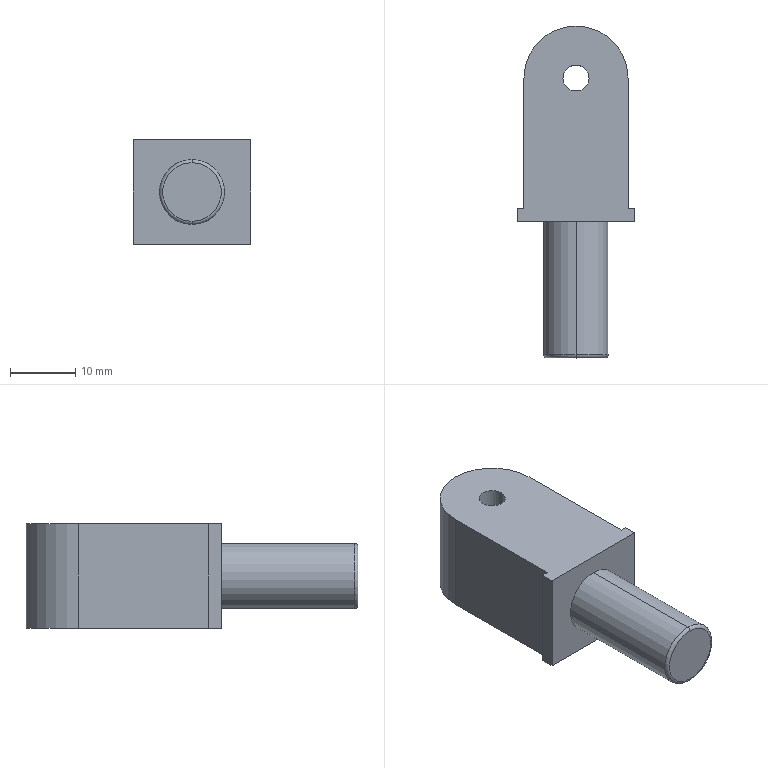Part | STEP file | Hinge middle | 1 solid | 17 faces | box 18 x 51 x 16 mm | volume 8751 mm3 | plane 10 | cylinder 5 | torus 2 | commonest cylinder face diameters 4 x2 10 x2 16 x1
STEP:
#1=CARTESIAN_POINT('',(0.,0.,0.));
#2=DIRECTION('',(0.,0.,1.));
#3=DIRECTION('',(1.,0.,0.));
#4=AXIS2_PLACEMENT_3D('',#1,#2,#3);
#5=CARTESIAN_POINT('',(0.,0.,-4.5));
#6=VERTEX_POINT('',#5);
#7=CARTESIAN_POINT('',(0.,0.,4.5));
#8=VERTEX_POINT('',#7);
#9=CARTESIAN_POINT('',(0.,0.,0.));
#10=DIRECTION('',(0.,-1.,0.));
#11=DIRECTION('',(0.,0.,1.));
#12=AXIS2_PLACEMENT_3D('',#9,#10,#11);
#13=CIRCLE('',#12,4.5);
#14=CARTESIAN_POINT('',(0.,0.5,0.));
#15=DIRECTION('',(0.,1.,0.));
#16=DIRECTION('',(0.,0.,1.));
#17=AXIS2_PLACEMENT_3D('',#14,#15,#16);
#18=TOROIDAL_SURFACE('',#17,4.5,0.5);
#19=CARTESIAN_POINT('',(6.283,4.712));
#20=DIRECTION('',(-1.,0.));
#21=VECTOR('',#20,1.);
#22=LINE('',#19,#21);
#23=(GEOMETRIC_REPRESENTATION_CONTEXT(2)PARAMETRIC_REPRESENTATION_CONTEXT()REPRESENTATION_CONTEXT('',''));
#24=DEFINITIONAL_REPRESENTATION('',(#22),#23);
#25=PCURVE('',#18,#24);
#26=CARTESIAN_POINT('',(0.,0.,0.));
#27=DIRECTION('',(0.,1.,0.));
#28=DIRECTION('',(0.,0.,1.));
#29=AXIS2_PLACEMENT_3D('',#26,#27,#28);
#30=PLANE('',#29);
#31=CARTESIAN_POINT('',(4.5,0.));
#32=CARTESIAN_POINT('',(4.5,-7.794));
#33=CARTESIAN_POINT('',(-2.25,-3.897));
#34=CARTESIAN_POINT('',(-9.,0.));
#35=CARTESIAN_POINT('',(-2.25,3.897));
#36=CARTESIAN_POINT('',(4.5,7.794));
#37=CARTESIAN_POINT('',(4.5,0.));
#38=(BOUNDED_CURVE()B_SPLINE_CURVE(2,(#31,#32,#33,#34,#35,#36,#37),.UNSPECIFIED.,.T.,.F.)B_SPLINE_CURVE_WITH_KNOTS((1,2,2,2,2,1),(-2.094,0.,2.094,4.189,6.283,8.378),.UNSPECIFIED.)CURVE()GEOMETRIC_REPRESENTATION_ITEM()RATIONAL_B_SPLINE_CURVE((1.,0.5,1.,0.5,1.,0.5,1.))REPRESENTATION_ITEM(''));
#39=(GEOMETRIC_REPRESENTATION_CONTEXT(2)PARAMETRIC_REPRESENTATION_CONTEXT()REPRESENTATION_CONTEXT('',''));
#40=DEFINITIONAL_REPRESENTATION('',(#38),#39);
#41=PCURVE('',#30,#40);
#42=SURFACE_CURVE('',#13,(#25,#41),.PCURVE_S1.);
#43=EDGE_CURVE('',#6,#8,#42,.T.);
#44=ORIENTED_EDGE('',*,*,#43,.F.);
#45=CARTESIAN_POINT('',(0.,0.5,-5.));
#46=VERTEX_POINT('',#45);
#47=CARTESIAN_POINT('',(0.,0.5,-4.5));
#48=DIRECTION('',(1.,0.,0.));
#49=DIRECTION('',(0.,0.,-1.));
#50=AXIS2_PLACEMENT_3D('',#47,#48,#49);
#51=CIRCLE('',#50,0.5);
#52=CARTESIAN_POINT('',(3.142,0.));
#53=DIRECTION('',(0.,1.));
#54=VECTOR('',#53,1.);
#55=LINE('',#52,#54);
#56=(GEOMETRIC_REPRESENTATION_CONTEXT(2)PARAMETRIC_REPRESENTATION_CONTEXT()REPRESENTATION_CONTEXT('',''));
#57=DEFINITIONAL_REPRESENTATION('',(#55),#56);
#58=PCURVE('',#18,#57);
#59=CARTESIAN_POINT('',(0.,0.5,0.));
#60=DIRECTION('',(0.,1.,0.));
#61=DIRECTION('',(0.,0.,1.));
#62=AXIS2_PLACEMENT_3D('',#59,#60,#61);
#63=TOROIDAL_SURFACE('',#62,4.5,0.5);
#64=CARTESIAN_POINT('',(3.142,0.));
#65=DIRECTION('',(0.,1.));
#66=VECTOR('',#65,1.);
#67=LINE('',#64,#66);
#68=(GEOMETRIC_REPRESENTATION_CONTEXT(2)PARAMETRIC_REPRESENTATION_CONTEXT()REPRESENTATION_CONTEXT('',''));
#69=DEFINITIONAL_REPRESENTATION('',(#67),#68);
#70=PCURVE('',#63,#69);
#71=SURFACE_CURVE('',#51,(#58,#70),.PCURVE_S1.);
#72=EDGE_CURVE('',#6,#46,#71,.T.);
#73=ORIENTED_EDGE('',*,*,#72,.T.);
#74=CARTESIAN_POINT('',(0.,0.5,5.));
#75=VERTEX_POINT('',#74);
#76=CARTESIAN_POINT('',(0.,0.5,0.));
#77=DIRECTION('',(0.,1.,0.));
#78=DIRECTION('',(0.,0.,1.));
#79=AXIS2_PLACEMENT_3D('',#76,#77,#78);
#80=CIRCLE('',#79,5.);
#81=CARTESIAN_POINT('',(0.,6.283));
#82=DIRECTION('',(1.,0.));
#83=VECTOR('',#82,1.);
#84=LINE('',#81,#83);
#85=(GEOMETRIC_REPRESENTATION_CONTEXT(2)PARAMETRIC_REPRESENTATION_CONTEXT()REPRESENTATION_CONTEXT('',''));
#86=DEFINITIONAL_REPRESENTATION('',(#84),#85);
#87=PCURVE('',#18,#86);
#88=CARTESIAN_POINT('',(0.,21.,0.));
#89=DIRECTION('',(0.,-1.,0.));
#90=DIRECTION('',(0.,0.,-1.));
#91=AXIS2_PLACEMENT_3D('',#88,#89,#90);
#92=CYLINDRICAL_SURFACE('',#91,5.);
#93=CARTESIAN_POINT('',(3.142,20.5));
#94=DIRECTION('',(-1.,0.));
#95=VECTOR('',#94,1.);
#96=LINE('',#93,#95);
#97=(GEOMETRIC_REPRESENTATION_CONTEXT(2)PARAMETRIC_REPRESENTATION_CONTEXT()REPRESENTATION_CONTEXT('',''));
#98=DEFINITIONAL_REPRESENTATION('',(#96),#97);
#99=PCURVE('',#92,#98);
#100=SURFACE_CURVE('',#80,(#87,#99),.PCURVE_S1.);
#101=EDGE_CURVE('',#75,#46,#100,.T.);
#102=ORIENTED_EDGE('',*,*,#101,.F.);
#103=CARTESIAN_POINT('',(0.,0.5,4.5));
#104=DIRECTION('',(-1.,0.,0.));
#105=DIRECTION('',(0.,0.,1.));
#106=AXIS2_PLACEMENT_3D('',#103,#104,#105);
#107=CIRCLE('',#106,0.5);
#108=CARTESIAN_POINT('',(0.,0.));
#109=DIRECTION('',(0.,1.));
#110=VECTOR('',#109,1.);
#111=LINE('',#108,#110);
#112=(GEOMETRIC_REPRESENTATION_CONTEXT(2)PARAMETRIC_REPRESENTATION_CONTEXT()REPRESENTATION_CONTEXT('',''));
#113=DEFINITIONAL_REPRESENTATION('',(#111),#112);
#114=PCURVE('',#18,#113);
#115=CARTESIAN_POINT('',(6.283,0.));
#116=DIRECTION('',(0.,1.));
#117=VECTOR('',#116,1.);
#118=LINE('',#115,#117);
#119=(GEOMETRIC_REPRESENTATION_CONTEXT(2)PARAMETRIC_REPRESENTATION_CONTEXT()REPRESENTATION_CONTEXT('',''));
#120=DEFINITIONAL_REPRESENTATION('',(#118),#119);
#121=PCURVE('',#63,#120);
#122=SURFACE_CURVE('',#107,(#114,#121),.PCURVE_S1.);
#123=EDGE_CURVE('',#8,#75,#122,.T.);
#124=ORIENTED_EDGE('',*,*,#123,.F.);
#125=EDGE_LOOP('',(#44,#73,#102,#124));
#126=FACE_BOUND('',#125,.T.);
#127=ADVANCED_FACE('',(#126),#18,.T.);
#128=CARTESIAN_POINT('',(-2.,43.,8.));
#129=VERTEX_POINT('',#128);
#130=CARTESIAN_POINT('',(-2.,43.,-8.));
#131=VERTEX_POINT('',#130);
#132=CARTESIAN_POINT('',(-2.,43.,8.));
#133=DIRECTION('',(0.,0.,-1.));
#134=VECTOR('',#133,1.);
#135=LINE('',#132,#134);
#136=CARTESIAN_POINT('',(0.,43.,8.));
#137=DIRECTION('',(0.,0.,-1.));
#138=DIRECTION('',(-1.,0.,0.));
#139=AXIS2_PLACEMENT_3D('',#136,#137,#138);
#140=CYLINDRICAL_SURFACE('',#139,2.);
#141=CARTESIAN_POINT('',(6.283,0.));
#142=DIRECTION('',(0.,1.));
#143=VECTOR('',#142,1.);
#144=LINE('',#141,#143);
#145=(GEOMETRIC_REPRESENTATION_CONTEXT(2)PARAMETRIC_REPRESENTATION_CONTEXT()REPRESENTATION_CONTEXT('',''));
#146=DEFINITIONAL_REPRESENTATION('',(#144),#145);
#147=PCURVE('',#140,#146);
#148=CARTESIAN_POINT('',(0.,43.,8.));
#149=DIRECTION('',(0.,0.,-1.));
#150=DIRECTION('',(-1.,0.,0.));
#151=AXIS2_PLACEMENT_3D('',#148,#149,#150);
#152=CYLINDRICAL_SURFACE('',#151,2.);
#153=CARTESIAN_POINT('',(0.,0.));
#154=DIRECTION('',(0.,1.));
#155=VECTOR('',#154,1.);
#156=LINE('',#153,#155);
#157=(GEOMETRIC_REPRESENTATION_CONTEXT(2)PARAMETRIC_REPRESENTATION_CONTEXT()REPRESENTATION_CONTEXT('',''));
#158=DEFINITIONAL_REPRESENTATION('',(#156),#157);
#159=PCURVE('',#152,#158);
#160=SURFACE_CURVE('',#135,(#147,#159),.PCURVE_S1.);
#161=EDGE_CURVE('',#129,#131,#160,.T.);
#162=ORIENTED_EDGE('',*,*,#161,.T.);
#163=CARTESIAN_POINT('',(2.,43.,-8.));
#164=VERTEX_POINT('',#163);
#165=CARTESIAN_POINT('',(0.,43.,-8.));
#166=DIRECTION('',(0.,0.,1.));
#167=DIRECTION('',(1.,0.,0.));
#168=AXIS2_PLACEMENT_3D('',#165,#166,#167);
#169=CIRCLE('',#168,2.);
#170=CARTESIAN_POINT('',(9.425,16.));
#171=DIRECTION('',(-1.,0.));
#172=VECTOR('',#171,1.);
#173=LINE('',#170,#172);
#174=(GEOMETRIC_REPRESENTATION_CONTEXT(2)PARAMETRIC_REPRESENTATION_CONTEXT()REPRESENTATION_CONTEXT('',''));
#175=DEFINITIONAL_REPRESENTATION('',(#173),#174);
#176=PCURVE('',#140,#175);
#177=CARTESIAN_POINT('',(-9.,23.,-8.));
#178=DIRECTION('',(0.,0.,1.));
#179=DIRECTION('',(1.,0.,0.));
#180=AXIS2_PLACEMENT_3D('',#177,#178,#179);
#181=PLANE('',#180);
#182=CARTESIAN_POINT('',(9.,20.));
#183=DIRECTION('',(1.,0.));
#184=AXIS2_PLACEMENT_2D('',#182,#183);
#185=CIRCLE('',#184,2.);
#186=(GEOMETRIC_REPRESENTATION_CONTEXT(2)PARAMETRIC_REPRESENTATION_CONTEXT()REPRESENTATION_CONTEXT('',''));
#187=DEFINITIONAL_REPRESENTATION('',(#185),#186);
#188=PCURVE('',#181,#187);
#189=SURFACE_CURVE('',#169,(#176,#188),.PCURVE_S1.);
#190=EDGE_CURVE('',#131,#164,#189,.T.);
#191=ORIENTED_EDGE('',*,*,#190,.T.);
#192=CARTESIAN_POINT('',(2.,43.,8.));
#193=VERTEX_POINT('',#192);
#194=CARTESIAN_POINT('',(2.,43.,8.));
#195=DIRECTION('',(0.,0.,-1.));
#196=VECTOR('',#195,1.);
#197=LINE('',#194,#196);
#198=CARTESIAN_POINT('',(3.142,0.));
#199=DIRECTION('',(0.,1.));
#200=VECTOR('',#199,1.);
#201=LINE('',#198,#200);
#202=(GEOMETRIC_REPRESENTATION_CONTEXT(2)PARAMETRIC_REPRESENTATION_CONTEXT()REPRESENTATION_CONTEXT('',''));
#203=DEFINITIONAL_REPRESENTATION('',(#201),#202);
#204=PCURVE('',#140,#203);
#205=CARTESIAN_POINT('',(3.142,0.));
#206=DIRECTION('',(0.,1.));
#207=VECTOR('',#206,1.);
#208=LINE('',#205,#207);
#209=(GEOMETRIC_REPRESENTATION_CONTEXT(2)PARAMETRIC_REPRESENTATION_CONTEXT()REPRESENTATION_CONTEXT('',''));
#210=DEFINITIONAL_REPRESENTATION('',(#208),#209);
#211=PCURVE('',#152,#210);
#212=SURFACE_CURVE('',#197,(#204,#211),.PCURVE_S1.);
#213=EDGE_CURVE('',#193,#164,#212,.T.);
#214=ORIENTED_EDGE('',*,*,#213,.F.);
#215=CARTESIAN_POINT('',(0.,43.,8.));
#216=DIRECTION('',(0.,0.,1.));
#217=DIRECTION('',(1.,0.,0.));
#218=AXIS2_PLACEMENT_3D('',#215,#216,#217);
#219=CIRCLE('',#218,2.);
#220=CARTESIAN_POINT('',(9.425,0.));
#221=DIRECTION('',(-1.,0.));
#222=VECTOR('',#221,1.);
#223=LINE('',#220,#222);
#224=(GEOMETRIC_REPRESENTATION_CONTEXT(2)PARAMETRIC_REPRESENTATION_CONTEXT()REPRESENTATION_CONTEXT('',''));
#225=DEFINITIONAL_REPRESENTATION('',(#223),#224);
#226=PCURVE('',#140,#225);
#227=CARTESIAN_POINT('',(-9.,23.,8.));
#228=DIRECTION('',(0.,0.,-1.));
#229=DIRECTION('',(-1.,0.,0.));
#230=AXIS2_PLACEMENT_3D('',#227,#228,#229);
#231=PLANE('',#230);
#232=CARTESIAN_POINT('',(-11.,20.));
#233=CARTESIAN_POINT('',(-11.,23.464));
#234=CARTESIAN_POINT('',(-8.,21.732));
#235=CARTESIAN_POINT('',(-5.,20.));
#236=CARTESIAN_POINT('',(-8.,18.268));
#237=CARTESIAN_POINT('',(-11.,16.536));
#238=CARTESIAN_POINT('',(-11.,20.));
#239=(BOUNDED_CURVE()B_SPLINE_CURVE(2,(#232,#233,#234,#235,#236,#237,#238),.UNSPECIFIED.,.T.,.F.)B_SPLINE_CURVE_WITH_KNOTS((1,2,2,2,2,1),(-2.094,0.,2.094,4.189,6.283,8.378),.UNSPECIFIED.)CURVE()GEOMETRIC_REPRESENTATION_ITEM()RATIONAL_B_SPLINE_CURVE((1.,0.5,1.,0.5,1.,0.5,1.))REPRESENTATION_ITEM(''));
#240=(GEOMETRIC_REPRESENTATION_CONTEXT(2)PARAMETRIC_REPRESENTATION_CONTEXT()REPRESENTATION_CONTEXT('',''));
#241=DEFINITIONAL_REPRESENTATION('',(#239),#240);
#242=PCURVE('',#231,#241);
#243=SURFACE_CURVE('',#219,(#226,#242),.PCURVE_S1.);
#244=EDGE_CURVE('',#129,#193,#243,.T.);
#245=ORIENTED_EDGE('',*,*,#244,.F.);
#246=EDGE_LOOP('',(#162,#191,#214,#245));
#247=FACE_BOUND('',#246,.F.);
#248=ADVANCED_FACE('',(#247),#140,.F.);
#249=CARTESIAN_POINT('',(0.,21.,5.));
#250=VERTEX_POINT('',#249);
#251=CARTESIAN_POINT('',(0.,21.,-5.));
#252=VERTEX_POINT('',#251);
#253=CARTESIAN_POINT('',(0.,21.,0.));
#254=DIRECTION('',(0.,1.,0.));
#255=DIRECTION('',(0.,0.,1.));
#256=AXIS2_PLACEMENT_3D('',#253,#254,#255);
#257=CIRCLE('',#256,5.);
#258=CARTESIAN_POINT('',(3.142,0.));
#259=DIRECTION('',(-1.,0.));
#260=VECTOR('',#259,1.);
#261=LINE('',#258,#260);
#262=(GEOMETRIC_REPRESENTATION_CONTEXT(2)PARAMETRIC_REPRESENTATION_CONTEXT()REPRESENTATION_CONTEXT('',''));
#263=DEFINITIONAL_REPRESENTATION('',(#261),#262);
#264=PCURVE('',#92,#263);
#265=CARTESIAN_POINT('',(0.,21.,0.));
#266=DIRECTION('',(0.,1.,0.));
#267=DIRECTION('',(0.,0.,1.));
#268=AXIS2_PLACEMENT_3D('',#265,#266,#267);
#269=PLANE('',#268);
#270=CARTESIAN_POINT('',(0.,0.));
#271=DIRECTION('',(1.,0.));
#272=AXIS2_PLACEMENT_2D('',#270,#271);
#273=CIRCLE('',#272,5.);
#274=(GEOMETRIC_REPRESENTATION_CONTEXT(2)PARAMETRIC_REPRESENTATION_CONTEXT()REPRESENTATION_CONTEXT('',''));
#275=DEFINITIONAL_REPRESENTATION('',(#273),#274);
#276=PCURVE('',#269,#275);
#277=SURFACE_CURVE('',#257,(#264,#276),.PCURVE_S1.);
#278=EDGE_CURVE('',#250,#252,#277,.T.);
#279=ORIENTED_EDGE('',*,*,#278,.F.);
#280=CARTESIAN_POINT('',(0.,21.,5.));
#281=DIRECTION('',(0.,-1.,0.));
#282=VECTOR('',#281,1.);
#283=LINE('',#280,#282);
#284=CARTESIAN_POINT('',(3.142,0.));
#285=DIRECTION('',(0.,1.));
#286=VECTOR('',#285,1.);
#287=LINE('',#284,#286);
#288=(GEOMETRIC_REPRESENTATION_CONTEXT(2)PARAMETRIC_REPRESENTATION_CONTEXT()REPRESENTATION_CONTEXT('',''));
#289=DEFINITIONAL_REPRESENTATION('',(#287),#288);
#290=PCURVE('',#92,#289);
#291=CARTESIAN_POINT('',(0.,21.,0.));
#292=DIRECTION('',(0.,-1.,0.));
#293=DIRECTION('',(0.,0.,-1.));
#294=AXIS2_PLACEMENT_3D('',#291,#292,#293);
#295=CYLINDRICAL_SURFACE('',#294,5.);
#296=CARTESIAN_POINT('',(3.142,0.));
#297=DIRECTION('',(0.,1.));
#298=VECTOR('',#297,1.);
#299=LINE('',#296,#298);
#300=(GEOMETRIC_REPRESENTATION_CONTEXT(2)PARAMETRIC_REPRESENTATION_CONTEXT()REPRESENTATION_CONTEXT('',''));
#301=DEFINITIONAL_REPRESENTATION('',(#299),#300);
#302=PCURVE('',#295,#301);
#303=SURFACE_CURVE('',#283,(#290,#302),.PCURVE_S1.);
#304=EDGE_CURVE('',#250,#75,#303,.T.);
#305=ORIENTED_EDGE('',*,*,#304,.T.);
#306=ORIENTED_EDGE('',*,*,#101,.T.);
#307=CARTESIAN_POINT('',(0.,21.,-5.));
#308=DIRECTION('',(0.,-1.,0.));
#309=VECTOR('',#308,1.);
#310=LINE('',#307,#309);
#311=CARTESIAN_POINT('',(0.,0.));
#312=DIRECTION('',(0.,1.));
#313=VECTOR('',#312,1.);
#314=LINE('',#311,#313);
#315=(GEOMETRIC_REPRESENTATION_CONTEXT(2)PARAMETRIC_REPRESENTATION_CONTEXT()REPRESENTATION_CONTEXT('',''));
#316=DEFINITIONAL_REPRESENTATION('',(#314),#315);
#317=PCURVE('',#92,#316);
#318=CARTESIAN_POINT('',(6.283,0.));
#319=DIRECTION('',(0.,1.));
#320=VECTOR('',#319,1.);
#321=LINE('',#318,#320);
#322=(GEOMETRIC_REPRESENTATION_CONTEXT(2)PARAMETRIC_REPRESENTATION_CONTEXT()REPRESENTATION_CONTEXT('',''));
#323=DEFINITIONAL_REPRESENTATION('',(#321),#322);
#324=PCURVE('',#295,#323);
#325=SURFACE_CURVE('',#310,(#317,#324),.PCURVE_S1.);
#326=EDGE_CURVE('',#252,#46,#325,.T.);
#327=ORIENTED_EDGE('',*,*,#326,.F.);
#328=EDGE_LOOP('',(#279,#305,#306,#327));
#329=FACE_BOUND('',#328,.T.);
#330=ADVANCED_FACE('',(#329),#92,.T.);
#331=CARTESIAN_POINT('',(-9.,23.,8.));
#332=VERTEX_POINT('',#331);
#333=CARTESIAN_POINT('',(-8.,23.,8.));
#334=VERTEX_POINT('',#333);
#335=CARTESIAN_POINT('',(-9.,23.,8.));
#336=DIRECTION('',(1.,0.,0.));
#337=VECTOR('',#336,1.);
#338=LINE('',#335,#337);
#339=CARTESIAN_POINT('',(0.,23.,0.));
#340=DIRECTION('',(0.,1.,0.));
#341=DIRECTION('',(0.,0.,1.));
#342=AXIS2_PLACEMENT_3D('',#339,#340,#341);
#343=PLANE('',#342);
#344=CARTESIAN_POINT('',(8.,-9.));
#345=DIRECTION('',(0.,1.));
#346=VECTOR('',#345,1.);
#347=LINE('',#344,#346);
#348=(GEOMETRIC_REPRESENTATION_CONTEXT(2)PARAMETRIC_REPRESENTATION_CONTEXT()REPRESENTATION_CONTEXT('',''));
#349=DEFINITIONAL_REPRESENTATION('',(#347),#348);
#350=PCURVE('',#343,#349);
#351=CARTESIAN_POINT('',(0.,0.));
#352=DIRECTION('',(-1.,0.));
#353=VECTOR('',#352,1.);
#354=LINE('',#351,#353);
#355=(GEOMETRIC_REPRESENTATION_CONTEXT(2)PARAMETRIC_REPRESENTATION_CONTEXT()REPRESENTATION_CONTEXT('',''));
#356=DEFINITIONAL_REPRESENTATION('',(#354),#355);
#357=PCURVE('',#231,#356);
#358=SURFACE_CURVE('',#338,(#350,#357),.PCURVE_S1.);
#359=EDGE_CURVE('',#332,#334,#358,.T.);
#360=ORIENTED_EDGE('',*,*,#359,.T.);
#361=CARTESIAN_POINT('',(-8.,23.,-8.));
#362=VERTEX_POINT('',#361);
#363=CARTESIAN_POINT('',(-8.,23.,8.));
#364=DIRECTION('',(0.,0.,-1.));
#365=VECTOR('',#364,1.);
#366=LINE('',#363,#365);
#367=CARTESIAN_POINT('',(8.,-8.));
#368=DIRECTION('',(-1.,0.));
#369=VECTOR('',#368,1.);
#370=LINE('',#367,#369);
#371=(GEOMETRIC_REPRESENTATION_CONTEXT(2)PARAMETRIC_REPRESENTATION_CONTEXT()REPRESENTATION_CONTEXT('',''));
#372=DEFINITIONAL_REPRESENTATION('',(#370),#371);
#373=PCURVE('',#343,#372);
#374=CARTESIAN_POINT('',(-8.,23.,8.));
#375=DIRECTION('',(1.,0.,0.));
#376=DIRECTION('',(0.,0.,-1.));
#377=AXIS2_PLACEMENT_3D('',#374,#375,#376);
#378=PLANE('',#377);
#379=CARTESIAN_POINT('',(0.,0.));
#380=DIRECTION('',(1.,0.));
#381=VECTOR('',#380,1.);
#382=LINE('',#379,#381);
#383=(GEOMETRIC_REPRESENTATION_CONTEXT(2)PARAMETRIC_REPRESENTATION_CONTEXT()REPRESENTATION_CONTEXT('',''));
#384=DEFINITIONAL_REPRESENTATION('',(#382),#383);
#385=PCURVE('',#378,#384);
#386=SURFACE_CURVE('',#366,(#373,#385),.PCURVE_S1.);
#387=EDGE_CURVE('',#334,#362,#386,.T.);
#388=ORIENTED_EDGE('',*,*,#387,.T.);
#389=CARTESIAN_POINT('',(-9.,23.,-8.));
#390=VERTEX_POINT('',#389);
#391=CARTESIAN_POINT('',(-9.,23.,-8.));
#392=DIRECTION('',(-1.,0.,0.));
#393=VECTOR('',#392,1.);
#394=LINE('',#391,#393);
#395=CARTESIAN_POINT('',(-8.,-9.));
#396=DIRECTION('',(0.,-1.));
#397=VECTOR('',#396,1.);
#398=LINE('',#395,#397);
#399=(GEOMETRIC_REPRESENTATION_CONTEXT(2)PARAMETRIC_REPRESENTATION_CONTEXT()REPRESENTATION_CONTEXT('',''));
#400=DEFINITIONAL_REPRESENTATION('',(#398),#399);
#401=PCURVE('',#343,#400);
#402=CARTESIAN_POINT('',(0.,0.));
#403=DIRECTION('',(-1.,0.));
#404=VECTOR('',#403,1.);
#405=LINE('',#402,#404);
#406=(GEOMETRIC_REPRESENTATION_CONTEXT(2)PARAMETRIC_REPRESENTATION_CONTEXT()REPRESENTATION_CONTEXT('',''));
#407=DEFINITIONAL_REPRESENTATION('',(#405),#406);
#408=PCURVE('',#181,#407);
#409=SURFACE_CURVE('',#394,(#401,#408),.PCURVE_S1.);
#410=EDGE_CURVE('',#362,#390,#409,.T.);
#411=ORIENTED_EDGE('',*,*,#410,.T.);
#412=CARTESIAN_POINT('',(-9.,23.,-8.));
#413=DIRECTION('',(0.,0.,1.));
#414=VECTOR('',#413,1.);
#415=LINE('',#412,#414);
#416=CARTESIAN_POINT('',(-8.,-9.));
#417=DIRECTION('',(1.,0.));
#418=VECTOR('',#417,1.);
#419=LINE('',#416,#418);
#420=(GEOMETRIC_REPRESENTATION_CONTEXT(2)PARAMETRIC_REPRESENTATION_CONTEXT()REPRESENTATION_CONTEXT('',''));
#421=DEFINITIONAL_REPRESENTATION('',(#419),#420);
#422=PCURVE('',#343,#421);
#423=CARTESIAN_POINT('',(-9.,23.,-8.));
#424=DIRECTION('',(1.,0.,0.));
#425=DIRECTION('',(0.,0.,-1.));
#426=AXIS2_PLACEMENT_3D('',#423,#424,#425);
#427=PLANE('',#426);
#428=CARTESIAN_POINT('',(0.,0.));
#429=DIRECTION('',(-1.,0.));
#430=VECTOR('',#429,1.);
#431=LINE('',#428,#430);
#432=(GEOMETRIC_REPRESENTATION_CONTEXT(2)PARAMETRIC_REPRESENTATION_CONTEXT()REPRESENTATION_CONTEXT('',''));
#433=DEFINITIONAL_REPRESENTATION('',(#431),#432);
#434=PCURVE('',#427,#433);
#435=SURFACE_CURVE('',#415,(#422,#434),.PCURVE_S1.);
#436=EDGE_CURVE('',#390,#332,#435,.T.);
#437=ORIENTED_EDGE('',*,*,#436,.T.);
#438=EDGE_LOOP('',(#360,#388,#411,#437));
#439=FACE_BOUND('',#438,.T.);
#440=ADVANCED_FACE('',(#439),#343,.T.);
#441=ORIENTED_EDGE('',*,*,#304,.F.);
#442=CARTESIAN_POINT('',(0.,21.,0.));
#443=DIRECTION('',(0.,1.,0.));
#444=DIRECTION('',(0.,0.,1.));
#445=AXIS2_PLACEMENT_3D('',#442,#443,#444);
#446=CIRCLE('',#445,5.);
#447=CARTESIAN_POINT('',(9.425,0.));
#448=DIRECTION('',(-1.,0.));
#449=VECTOR('',#448,1.);
#450=LINE('',#447,#449);
#451=(GEOMETRIC_REPRESENTATION_CONTEXT(2)PARAMETRIC_REPRESENTATION_CONTEXT()REPRESENTATION_CONTEXT('',''));
#452=DEFINITIONAL_REPRESENTATION('',(#450),#451);
#453=PCURVE('',#295,#452);
#454=CARTESIAN_POINT('',(0.,0.));
#455=DIRECTION('',(1.,0.));
#456=AXIS2_PLACEMENT_2D('',#454,#455);
#457=CIRCLE('',#456,5.);
#458=(GEOMETRIC_REPRESENTATION_CONTEXT(2)PARAMETRIC_REPRESENTATION_CONTEXT()REPRESENTATION_CONTEXT('',''));
#459=DEFINITIONAL_REPRESENTATION('',(#457),#458);
#460=PCURVE('',#269,#459);
#461=SURFACE_CURVE('',#446,(#453,#460),.PCURVE_S1.);
#462=EDGE_CURVE('',#252,#250,#461,.T.);
#463=ORIENTED_EDGE('',*,*,#462,.F.);
#464=ORIENTED_EDGE('',*,*,#326,.T.);
#465=CARTESIAN_POINT('',(0.,0.5,0.));
#466=DIRECTION('',(0.,1.,0.));
#467=DIRECTION('',(0.,0.,1.));
#468=AXIS2_PLACEMENT_3D('',#465,#466,#467);
#469=CIRCLE('',#468,5.);
#470=CARTESIAN_POINT('',(9.425,20.5));
#471=DIRECTION('',(-1.,0.));
#472=VECTOR('',#471,1.);
#473=LINE('',#470,#472);
#474=(GEOMETRIC_REPRESENTATION_CONTEXT(2)PARAMETRIC_REPRESENTATION_CONTEXT()REPRESENTATION_CONTEXT('',''));
#475=DEFINITIONAL_REPRESENTATION('',(#473),#474);
#476=PCURVE('',#295,#475);
#477=CARTESIAN_POINT('',(0.,6.283));
#478=DIRECTION('',(1.,0.));
#479=VECTOR('',#478,1.);
#480=LINE('',#477,#479);
#481=(GEOMETRIC_REPRESENTATION_CONTEXT(2)PARAMETRIC_REPRESENTATION_CONTEXT()REPRESENTATION_CONTEXT('',''));
#482=DEFINITIONAL_REPRESENTATION('',(#480),#481);
#483=PCURVE('',#63,#482);
#484=SURFACE_CURVE('',#469,(#476,#483),.PCURVE_S1.);
#485=EDGE_CURVE('',#46,#75,#484,.T.);
#486=ORIENTED_EDGE('',*,*,#485,.T.);
#487=EDGE_LOOP('',(#441,#463,#464,#486));
#488=FACE_BOUND('',#487,.T.);
#489=ADVANCED_FACE('',(#488),#295,.T.);
#490=CARTESIAN_POINT('',(0.,0.,0.));
#491=DIRECTION('',(0.,-1.,0.));
#492=DIRECTION('',(0.,0.,1.));
#493=AXIS2_PLACEMENT_3D('',#490,#491,#492);
#494=CIRCLE('',#493,4.5);
#495=CARTESIAN_POINT('',(4.5,0.));
#496=CARTESIAN_POINT('',(4.5,-7.794));
#497=CARTESIAN_POINT('',(-2.25,-3.897));
#498=CARTESIAN_POINT('',(-9.,0.));
#499=CARTESIAN_POINT('',(-2.25,3.897));
#500=CARTESIAN_POINT('',(4.5,7.794));
#501=CARTESIAN_POINT('',(4.5,0.));
#502=(BOUNDED_CURVE()B_SPLINE_CURVE(2,(#495,#496,#497,#498,#499,#500,#501),.UNSPECIFIED.,.T.,.F.)B_SPLINE_CURVE_WITH_KNOTS((1,2,2,2,2,1),(-2.094,0.,2.094,4.189,6.283,8.378),.UNSPECIFIED.)CURVE()GEOMETRIC_REPRESENTATION_ITEM()RATIONAL_B_SPLINE_CURVE((1.,0.5,1.,0.5,1.,0.5,1.))REPRESENTATION_ITEM(''));
#503=(GEOMETRIC_REPRESENTATION_CONTEXT(2)PARAMETRIC_REPRESENTATION_CONTEXT()REPRESENTATION_CONTEXT('',''));
#504=DEFINITIONAL_REPRESENTATION('',(#502),#503);
#505=PCURVE('',#30,#504);
#506=CARTESIAN_POINT('',(6.283,4.712));
#507=DIRECTION('',(-1.,0.));
#508=VECTOR('',#507,1.);
#509=LINE('',#506,#508);
#510=(GEOMETRIC_REPRESENTATION_CONTEXT(2)PARAMETRIC_REPRESENTATION_CONTEXT()REPRESENTATION_CONTEXT('',''));
#511=DEFINITIONAL_REPRESENTATION('',(#509),#510);
#512=PCURVE('',#63,#511);
#513=SURFACE_CURVE('',#494,(#505,#512),.PCURVE_S1.);
#514=EDGE_CURVE('',#8,#6,#513,.T.);
#515=ORIENTED_EDGE('',*,*,#514,.T.);
#516=ORIENTED_EDGE('',*,*,#43,.T.);
#517=EDGE_LOOP('',(#515,#516));
#518=FACE_BOUND('',#517,.T.);
#519=ADVANCED_FACE('',(#518),#30,.F.);
#520=CARTESIAN_POINT('',(9.,21.,8.));
#521=VERTEX_POINT('',#520);
#522=CARTESIAN_POINT('',(9.,21.,-8.));
#523=VERTEX_POINT('',#522);
#524=CARTESIAN_POINT('',(9.,21.,-8.));
#525=DIRECTION('',(0.,0.,-1.));
#526=VECTOR('',#525,1.);
#527=LINE('',#524,#526);
#528=CARTESIAN_POINT('',(9.,23.,-8.));
#529=DIRECTION('',(-1.,0.,0.));
#530=DIRECTION('',(0.,0.,1.));
#531=AXIS2_PLACEMENT_3D('',#528,#529,#530);
#532=PLANE('',#531);
#533=CARTESIAN_POINT('',(0.,-2.));
#534=DIRECTION('',(-1.,0.));
#535=VECTOR('',#534,1.);
#536=LINE('',#533,#535);
#537=(GEOMETRIC_REPRESENTATION_CONTEXT(2)PARAMETRIC_REPRESENTATION_CONTEXT()REPRESENTATION_CONTEXT('',''));
#538=DEFINITIONAL_REPRESENTATION('',(#536),#537);
#539=PCURVE('',#532,#538);
#540=CARTESIAN_POINT('',(-8.,9.));
#541=DIRECTION('',(-1.,0.));
#542=VECTOR('',#541,1.);
#543=LINE('',#540,#542);
#544=(GEOMETRIC_REPRESENTATION_CONTEXT(2)PARAMETRIC_REPRESENTATION_CONTEXT()REPRESENTATION_CONTEXT('',''));
#545=DEFINITIONAL_REPRESENTATION('',(#543),#544);
#546=PCURVE('',#269,#545);
#547=SURFACE_CURVE('',#527,(#539,#546),.PCURVE_S1.);
#548=EDGE_CURVE('',#521,#523,#547,.T.);
#549=ORIENTED_EDGE('',*,*,#548,.T.);
#550=CARTESIAN_POINT('',(9.,23.,-8.));
#551=VERTEX_POINT('',#550);
#552=CARTESIAN_POINT('',(9.,23.,-8.));
#553=DIRECTION('',(0.,-1.,0.));
#554=VECTOR('',#553,1.);
#555=LINE('',#552,#554);
#556=CARTESIAN_POINT('',(0.,0.));
#557=DIRECTION('',(0.,-1.));
#558=VECTOR('',#557,1.);
#559=LINE('',#556,#558);
#560=(GEOMETRIC_REPRESENTATION_CONTEXT(2)PARAMETRIC_REPRESENTATION_CONTEXT()REPRESENTATION_CONTEXT('',''));
#561=DEFINITIONAL_REPRESENTATION('',(#559),#560);
#562=PCURVE('',#532,#561);
#563=CARTESIAN_POINT('',(18.,0.));
#564=DIRECTION('',(0.,-1.));
#565=VECTOR('',#564,1.);
#566=LINE('',#563,#565);
#567=(GEOMETRIC_REPRESENTATION_CONTEXT(2)PARAMETRIC_REPRESENTATION_CONTEXT()REPRESENTATION_CONTEXT('',''));
#568=DEFINITIONAL_REPRESENTATION('',(#566),#567);
#569=PCURVE('',#181,#568);
#570=SURFACE_CURVE('',#555,(#562,#569),.PCURVE_S1.);
#571=EDGE_CURVE('',#551,#523,#570,.T.);
#572=ORIENTED_EDGE('',*,*,#571,.F.);
#573=CARTESIAN_POINT('',(9.,23.,8.));
#574=VERTEX_POINT('',#573);
#575=CARTESIAN_POINT('',(9.,23.,-8.));
#576=DIRECTION('',(0.,0.,-1.));
#577=VECTOR('',#576,1.);
#578=LINE('',#575,#577);
#579=CARTESIAN_POINT('',(0.,0.));
#580=DIRECTION('',(-1.,0.));
#581=VECTOR('',#580,1.);
#582=LINE('',#579,#581);
#583=(GEOMETRIC_REPRESENTATION_CONTEXT(2)PARAMETRIC_REPRESENTATION_CONTEXT()REPRESENTATION_CONTEXT('',''));
#584=DEFINITIONAL_REPRESENTATION('',(#582),#583);
#585=PCURVE('',#532,#584);
#586=CARTESIAN_POINT('',(0.,23.,0.));
#587=DIRECTION('',(0.,1.,0.));
#588=DIRECTION('',(0.,0.,1.));
#589=AXIS2_PLACEMENT_3D('',#586,#587,#588);
#590=PLANE('',#589);
#591=CARTESIAN_POINT('',(-8.,9.));
#592=DIRECTION('',(-1.,0.));
#593=VECTOR('',#592,1.);
#594=LINE('',#591,#593);
#595=(GEOMETRIC_REPRESENTATION_CONTEXT(2)PARAMETRIC_REPRESENTATION_CONTEXT()REPRESENTATION_CONTEXT('',''));
#596=DEFINITIONAL_REPRESENTATION('',(#594),#595);
#597=PCURVE('',#590,#596);
#598=SURFACE_CURVE('',#578,(#585,#597),.PCURVE_S1.);
#599=EDGE_CURVE('',#574,#551,#598,.T.);
#600=ORIENTED_EDGE('',*,*,#599,.F.);
#601=CARTESIAN_POINT('',(9.,23.,8.));
#602=DIRECTION('',(0.,-1.,0.));
#603=VECTOR('',#602,1.);
#604=LINE('',#601,#603);
#605=CARTESIAN_POINT('',(16.,0.));
#606=DIRECTION('',(0.,-1.));
#607=VECTOR('',#606,1.);
#608=LINE('',#605,#607);
#609=(GEOMETRIC_REPRESENTATION_CONTEXT(2)PARAMETRIC_REPRESENTATION_CONTEXT()REPRESENTATION_CONTEXT('',''));
#610=DEFINITIONAL_REPRESENTATION('',(#608),#609);
#611=PCURVE('',#532,#610);
#612=CARTESIAN_POINT('',(-18.,0.));
#613=DIRECTION('',(0.,-1.));
#614=VECTOR('',#613,1.);
#615=LINE('',#612,#614);
#616=(GEOMETRIC_REPRESENTATION_CONTEXT(2)PARAMETRIC_REPRESENTATION_CONTEXT()REPRESENTATION_CONTEXT('',''));
#617=DEFINITIONAL_REPRESENTATION('',(#615),#616);
#618=PCURVE('',#231,#617);
#619=SURFACE_CURVE('',#604,(#611,#618),.PCURVE_S1.);
#620=EDGE_CURVE('',#574,#521,#619,.T.);
#621=ORIENTED_EDGE('',*,*,#620,.T.);
#622=EDGE_LOOP('',(#549,#572,#600,#621));
#623=FACE_BOUND('',#622,.T.);
#624=ADVANCED_FACE('',(#623),#532,.F.);
#625=CARTESIAN_POINT('',(-9.,21.,-8.));
#626=VERTEX_POINT('',#625);
#627=CARTESIAN_POINT('',(-9.,21.,-8.));
#628=DIRECTION('',(-1.,0.,0.));
#629=VECTOR('',#628,1.);
#630=LINE('',#627,#629);
#631=CARTESIAN_POINT('',(0.,-2.));
#632=DIRECTION('',(-1.,0.));
#633=VECTOR('',#632,1.);
#634=LINE('',#631,#633);
#635=(GEOMETRIC_REPRESENTATION_CONTEXT(2)PARAMETRIC_REPRESENTATION_CONTEXT()REPRESENTATION_CONTEXT('',''));
#636=DEFINITIONAL_REPRESENTATION('',(#634),#635);
#637=PCURVE('',#181,#636);
#638=CARTESIAN_POINT('',(-8.,-9.));
#639=DIRECTION('',(0.,-1.));
#640=VECTOR('',#639,1.);
#641=LINE('',#638,#640);
#642=(GEOMETRIC_REPRESENTATION_CONTEXT(2)PARAMETRIC_REPRESENTATION_CONTEXT()REPRESENTATION_CONTEXT('',''));
#643=DEFINITIONAL_REPRESENTATION('',(#641),#642);
#644=PCURVE('',#269,#643);
#645=SURFACE_CURVE('',#630,(#637,#644),.PCURVE_S1.);
#646=EDGE_CURVE('',#523,#626,#645,.T.);
#647=ORIENTED_EDGE('',*,*,#646,.T.);
#648=CARTESIAN_POINT('',(-9.,23.,-8.));
#649=DIRECTION('',(0.,-1.,0.));
#650=VECTOR('',#649,1.);
#651=LINE('',#648,#650);
#652=CARTESIAN_POINT('',(0.,0.));
#653=DIRECTION('',(0.,-1.));
#654=VECTOR('',#653,1.);
#655=LINE('',#652,#654);
#656=(GEOMETRIC_REPRESENTATION_CONTEXT(2)PARAMETRIC_REPRESENTATION_CONTEXT()REPRESENTATION_CONTEXT('',''));
#657=DEFINITIONAL_REPRESENTATION('',(#655),#656);
#658=PCURVE('',#181,#657);
#659=CARTESIAN_POINT('',(0.,0.));
#660=DIRECTION('',(0.,-1.));
#661=VECTOR('',#660,1.);
#662=LINE('',#659,#661);
#663=(GEOMETRIC_REPRESENTATION_CONTEXT(2)PARAMETRIC_REPRESENTATION_CONTEXT()REPRESENTATION_CONTEXT('',''));
#664=DEFINITIONAL_REPRESENTATION('',(#662),#663);
#665=PCURVE('',#427,#664);
#666=SURFACE_CURVE('',#651,(#658,#665),.PCURVE_S1.);
#667=EDGE_CURVE('',#390,#626,#666,.T.);
#668=ORIENTED_EDGE('',*,*,#667,.F.);
#669=ORIENTED_EDGE('',*,*,#410,.F.);
#670=CARTESIAN_POINT('',(-8.,43.,-8.));
#671=VERTEX_POINT('',#670);
#672=CARTESIAN_POINT('',(-8.,23.,-8.));
#673=DIRECTION('',(0.,-1.,0.));
#674=VECTOR('',#673,1.);
#675=LINE('',#672,#674);
#676=CARTESIAN_POINT('',(1.,0.));
#677=DIRECTION('',(0.,-1.));
#678=VECTOR('',#677,1.);
#679=LINE('',#676,#678);
#680=(GEOMETRIC_REPRESENTATION_CONTEXT(2)PARAMETRIC_REPRESENTATION_CONTEXT()REPRESENTATION_CONTEXT('',''));
#681=DEFINITIONAL_REPRESENTATION('',(#679),#680);
#682=PCURVE('',#181,#681);
#683=CARTESIAN_POINT('',(16.,0.));
#684=DIRECTION('',(0.,-1.));
#685=VECTOR('',#684,1.);
#686=LINE('',#683,#685);
#687=(GEOMETRIC_REPRESENTATION_CONTEXT(2)PARAMETRIC_REPRESENTATION_CONTEXT()REPRESENTATION_CONTEXT('',''));
#688=DEFINITIONAL_REPRESENTATION('',(#686),#687);
#689=PCURVE('',#378,#688);
#690=SURFACE_CURVE('',#675,(#682,#689),.PCURVE_S1.);
#691=EDGE_CURVE('',#671,#362,#690,.T.);
#692=ORIENTED_EDGE('',*,*,#691,.F.);
#693=CARTESIAN_POINT('',(8.,43.,-8.));
#694=VERTEX_POINT('',#693);
#695=CARTESIAN_POINT('',(0.,43.,-8.));
#696=DIRECTION('',(0.,0.,1.));
#697=DIRECTION('',(-1.,0.,0.));
#698=AXIS2_PLACEMENT_3D('',#695,#696,#697);
#699=CIRCLE('',#698,8.);
#700=CARTESIAN_POINT('',(9.,20.));
#701=DIRECTION('',(-1.,0.));
#702=AXIS2_PLACEMENT_2D('',#700,#701);
#703=CIRCLE('',#702,8.);
#704=(GEOMETRIC_REPRESENTATION_CONTEXT(2)PARAMETRIC_REPRESENTATION_CONTEXT()REPRESENTATION_CONTEXT('',''));
#705=DEFINITIONAL_REPRESENTATION('',(#703),#704);
#706=PCURVE('',#181,#705);
#707=CARTESIAN_POINT('',(0.,43.,8.));
#708=DIRECTION('',(0.,0.,-1.));
#709=DIRECTION('',(-1.,0.,0.));
#710=AXIS2_PLACEMENT_3D('',#707,#708,#709);
#711=CYLINDRICAL_SURFACE('',#710,8.);
#712=CARTESIAN_POINT('',(6.283,16.));
#713=DIRECTION('',(-1.,0.));
#714=VECTOR('',#713,1.);
#715=LINE('',#712,#714);
#716=(GEOMETRIC_REPRESENTATION_CONTEXT(2)PARAMETRIC_REPRESENTATION_CONTEXT()REPRESENTATION_CONTEXT('',''));
#717=DEFINITIONAL_REPRESENTATION('',(#715),#716);
#718=PCURVE('',#711,#717);
#719=SURFACE_CURVE('',#699,(#706,#718),.PCURVE_S1.);
#720=EDGE_CURVE('',#694,#671,#719,.T.);
#721=ORIENTED_EDGE('',*,*,#720,.F.);
#722=CARTESIAN_POINT('',(8.,23.,-8.));
#723=VERTEX_POINT('',#722);
#724=CARTESIAN_POINT('',(8.,23.,-8.));
#725=DIRECTION('',(0.,1.,0.));
#726=VECTOR('',#725,1.);
#727=LINE('',#724,#726);
#728=CARTESIAN_POINT('',(17.,0.));
#729=DIRECTION('',(0.,1.));
#730=VECTOR('',#729,1.);
#731=LINE('',#728,#730);
#732=(GEOMETRIC_REPRESENTATION_CONTEXT(2)PARAMETRIC_REPRESENTATION_CONTEXT()REPRESENTATION_CONTEXT('',''));
#733=DEFINITIONAL_REPRESENTATION('',(#731),#732);
#734=PCURVE('',#181,#733);
#735=CARTESIAN_POINT('',(8.,23.,8.));
#736=DIRECTION('',(-1.,0.,0.));
#737=DIRECTION('',(0.,0.,1.));
#738=AXIS2_PLACEMENT_3D('',#735,#736,#737);
#739=PLANE('',#738);
#740=CARTESIAN_POINT('',(-16.,0.));
#741=DIRECTION('',(0.,1.));
#742=VECTOR('',#741,1.);
#743=LINE('',#740,#742);
#744=(GEOMETRIC_REPRESENTATION_CONTEXT(2)PARAMETRIC_REPRESENTATION_CONTEXT()REPRESENTATION_CONTEXT('',''));
#745=DEFINITIONAL_REPRESENTATION('',(#743),#744);
#746=PCURVE('',#739,#745);
#747=SURFACE_CURVE('',#727,(#734,#746),.PCURVE_S1.);
#748=EDGE_CURVE('',#723,#694,#747,.T.);
#749=ORIENTED_EDGE('',*,*,#748,.F.);
#750=CARTESIAN_POINT('',(-9.,23.,-8.));
#751=DIRECTION('',(-1.,0.,0.));
#752=VECTOR('',#751,1.);
#753=LINE('',#750,#752);
#754=CARTESIAN_POINT('',(0.,0.));
#755=DIRECTION('',(-1.,0.));
#756=VECTOR('',#755,1.);
#757=LINE('',#754,#756);
#758=(GEOMETRIC_REPRESENTATION_CONTEXT(2)PARAMETRIC_REPRESENTATION_CONTEXT()REPRESENTATION_CONTEXT('',''));
#759=DEFINITIONAL_REPRESENTATION('',(#757),#758);
#760=PCURVE('',#181,#759);
#761=CARTESIAN_POINT('',(-8.,-9.));
#762=DIRECTION('',(0.,-1.));
#763=VECTOR('',#762,1.);
#764=LINE('',#761,#763);
#765=(GEOMETRIC_REPRESENTATION_CONTEXT(2)PARAMETRIC_REPRESENTATION_CONTEXT()REPRESENTATION_CONTEXT('',''));
#766=DEFINITIONAL_REPRESENTATION('',(#764),#765);
#767=PCURVE('',#590,#766);
#768=SURFACE_CURVE('',#753,(#760,#767),.PCURVE_S1.);
#769=EDGE_CURVE('',#551,#723,#768,.T.);
#770=ORIENTED_EDGE('',*,*,#769,.F.);
#771=ORIENTED_EDGE('',*,*,#571,.T.);
#772=EDGE_LOOP('',(#647,#668,#669,#692,#721,#749,#770,#771));
#773=FACE_BOUND('',#772,.T.);
#774=ORIENTED_EDGE('',*,*,#190,.T.);
#775=CARTESIAN_POINT('',(0.,43.,-8.));
#776=DIRECTION('',(0.,0.,1.));
#777=DIRECTION('',(1.,0.,0.));
#778=AXIS2_PLACEMENT_3D('',#775,#776,#777);
#779=CIRCLE('',#778,2.);
#780=CARTESIAN_POINT('',(9.,20.));
#781=DIRECTION('',(1.,0.));
#782=AXIS2_PLACEMENT_2D('',#780,#781);
#783=CIRCLE('',#782,2.);
#784=(GEOMETRIC_REPRESENTATION_CONTEXT(2)PARAMETRIC_REPRESENTATION_CONTEXT()REPRESENTATION_CONTEXT('',''));
#785=DEFINITIONAL_REPRESENTATION('',(#783),#784);
#786=PCURVE('',#181,#785);
#787=CARTESIAN_POINT('',(3.142,16.));
#788=DIRECTION('',(-1.,0.));
#789=VECTOR('',#788,1.);
#790=LINE('',#787,#789);
#791=(GEOMETRIC_REPRESENTATION_CONTEXT(2)PARAMETRIC_REPRESENTATION_CONTEXT()REPRESENTATION_CONTEXT('',''));
#792=DEFINITIONAL_REPRESENTATION('',(#790),#791);
#793=PCURVE('',#152,#792);
#794=SURFACE_CURVE('',#779,(#786,#793),.PCURVE_S1.);
#795=EDGE_CURVE('',#164,#131,#794,.T.);
#796=ORIENTED_EDGE('',*,*,#795,.T.);
#797=EDGE_LOOP('',(#774,#796));
#798=FACE_BOUND('',#797,.T.);
#799=ADVANCED_FACE('',(#773,#798),#181,.F.);
#800=CARTESIAN_POINT('',(-9.,21.,8.));
#801=VERTEX_POINT('',#800);
#802=CARTESIAN_POINT('',(-9.,21.,-8.));
#803=DIRECTION('',(0.,0.,1.));
#804=VECTOR('',#803,1.);
#805=LINE('',#802,#804);
#806=CARTESIAN_POINT('',(0.,-2.));
#807=DIRECTION('',(-1.,0.));
#808=VECTOR('',#807,1.);
#809=LINE('',#806,#808);
#810=(GEOMETRIC_REPRESENTATION_CONTEXT(2)PARAMETRIC_REPRESENTATION_CONTEXT()REPRESENTATION_CONTEXT('',''));
#811=DEFINITIONAL_REPRESENTATION('',(#809),#810);
#812=PCURVE('',#427,#811);
#813=CARTESIAN_POINT('',(-8.,-9.));
#814=DIRECTION('',(1.,0.));
#815=VECTOR('',#814,1.);
#816=LINE('',#813,#815);
#817=(GEOMETRIC_REPRESENTATION_CONTEXT(2)PARAMETRIC_REPRESENTATION_CONTEXT()REPRESENTATION_CONTEXT('',''));
#818=DEFINITIONAL_REPRESENTATION('',(#816),#817);
#819=PCURVE('',#269,#818);
#820=SURFACE_CURVE('',#805,(#812,#819),.PCURVE_S1.);
#821=EDGE_CURVE('',#626,#801,#820,.T.);
#822=ORIENTED_EDGE('',*,*,#821,.T.);
#823=CARTESIAN_POINT('',(-9.,23.,8.));
#824=DIRECTION('',(0.,-1.,0.));
#825=VECTOR('',#824,1.);
#826=LINE('',#823,#825);
#827=CARTESIAN_POINT('',(-16.,0.));
#828=DIRECTION('',(0.,-1.));
#829=VECTOR('',#828,1.);
#830=LINE('',#827,#829);
#831=(GEOMETRIC_REPRESENTATION_CONTEXT(2)PARAMETRIC_REPRESENTATION_CONTEXT()REPRESENTATION_CONTEXT('',''));
#832=DEFINITIONAL_REPRESENTATION('',(#830),#831);
#833=PCURVE('',#427,#832);
#834=CARTESIAN_POINT('',(0.,0.));
#835=DIRECTION('',(0.,-1.));
#836=VECTOR('',#835,1.);
#837=LINE('',#834,#836);
#838=(GEOMETRIC_REPRESENTATION_CONTEXT(2)PARAMETRIC_REPRESENTATION_CONTEXT()REPRESENTATION_CONTEXT('',''));
#839=DEFINITIONAL_REPRESENTATION('',(#837),#838);
#840=PCURVE('',#231,#839);
#841=SURFACE_CURVE('',#826,(#833,#840),.PCURVE_S1.);
#842=EDGE_CURVE('',#332,#801,#841,.T.);
#843=ORIENTED_EDGE('',*,*,#842,.F.);
#844=ORIENTED_EDGE('',*,*,#436,.F.);
#845=ORIENTED_EDGE('',*,*,#667,.T.);
#846=EDGE_LOOP('',(#822,#843,#844,#845));
#847=FACE_BOUND('',#846,.T.);
#848=ADVANCED_FACE('',(#847),#427,.F.);
#849=CARTESIAN_POINT('',(-9.,21.,8.));
#850=DIRECTION('',(1.,0.,0.));
#851=VECTOR('',#850,1.);
#852=LINE('',#849,#851);
#853=CARTESIAN_POINT('',(0.,-2.));
#854=DIRECTION('',(-1.,0.));
#855=VECTOR('',#854,1.);
#856=LINE('',#853,#855);
#857=(GEOMETRIC_REPRESENTATION_CONTEXT(2)PARAMETRIC_REPRESENTATION_CONTEXT()REPRESENTATION_CONTEXT('',''));
#858=DEFINITIONAL_REPRESENTATION('',(#856),#857);
#859=PCURVE('',#231,#858);
#860=CARTESIAN_POINT('',(8.,-9.));
#861=DIRECTION('',(0.,1.));
#862=VECTOR('',#861,1.);
#863=LINE('',#860,#862);
#864=(GEOMETRIC_REPRESENTATION_CONTEXT(2)PARAMETRIC_REPRESENTATION_CONTEXT()REPRESENTATION_CONTEXT('',''));
#865=DEFINITIONAL_REPRESENTATION('',(#863),#864);
#866=PCURVE('',#269,#865);
#867=SURFACE_CURVE('',#852,(#859,#866),.PCURVE_S1.);
#868=EDGE_CURVE('',#801,#521,#867,.T.);
#869=ORIENTED_EDGE('',*,*,#868,.T.);
#870=ORIENTED_EDGE('',*,*,#620,.F.);
#871=CARTESIAN_POINT('',(8.,23.,8.));
#872=VERTEX_POINT('',#871);
#873=CARTESIAN_POINT('',(-9.,23.,8.));
#874=DIRECTION('',(1.,0.,0.));
#875=VECTOR('',#874,1.);
#876=LINE('',#873,#875);
#877=CARTESIAN_POINT('',(0.,0.));
#878=DIRECTION('',(-1.,0.));
#879=VECTOR('',#878,1.);
#880=LINE('',#877,#879);
#881=(GEOMETRIC_REPRESENTATION_CONTEXT(2)PARAMETRIC_REPRESENTATION_CONTEXT()REPRESENTATION_CONTEXT('',''));
#882=DEFINITIONAL_REPRESENTATION('',(#880),#881);
#883=PCURVE('',#231,#882);
#884=CARTESIAN_POINT('',(8.,-9.));
#885=DIRECTION('',(0.,1.));
#886=VECTOR('',#885,1.);
#887=LINE('',#884,#886);
#888=(GEOMETRIC_REPRESENTATION_CONTEXT(2)PARAMETRIC_REPRESENTATION_CONTEXT()REPRESENTATION_CONTEXT('',''));
#889=DEFINITIONAL_REPRESENTATION('',(#887),#888);
#890=PCURVE('',#590,#889);
#891=SURFACE_CURVE('',#876,(#883,#890),.PCURVE_S1.);
#892=EDGE_CURVE('',#872,#574,#891,.T.);
#893=ORIENTED_EDGE('',*,*,#892,.F.);
#894=CARTESIAN_POINT('',(8.,43.,8.));
#895=VERTEX_POINT('',#894);
#896=CARTESIAN_POINT('',(8.,23.,8.));
#897=DIRECTION('',(0.,1.,0.));
#898=VECTOR('',#897,1.);
#899=LINE('',#896,#898);
#900=CARTESIAN_POINT('',(-17.,0.));
#901=DIRECTION('',(0.,1.));
#902=VECTOR('',#901,1.);
#903=LINE('',#900,#902);
#904=(GEOMETRIC_REPRESENTATION_CONTEXT(2)PARAMETRIC_REPRESENTATION_CONTEXT()REPRESENTATION_CONTEXT('',''));
#905=DEFINITIONAL_REPRESENTATION('',(#903),#904);
#906=PCURVE('',#231,#905);
#907=CARTESIAN_POINT('',(0.,0.));
#908=DIRECTION('',(0.,1.));
#909=VECTOR('',#908,1.);
#910=LINE('',#907,#909);
#911=(GEOMETRIC_REPRESENTATION_CONTEXT(2)PARAMETRIC_REPRESENTATION_CONTEXT()REPRESENTATION_CONTEXT('',''));
#912=DEFINITIONAL_REPRESENTATION('',(#910),#911);
#913=PCURVE('',#739,#912);
#914=SURFACE_CURVE('',#899,(#906,#913),.PCURVE_S1.);
#915=EDGE_CURVE('',#872,#895,#914,.T.);
#916=ORIENTED_EDGE('',*,*,#915,.T.);
#917=CARTESIAN_POINT('',(-8.,43.,8.));
#918=VERTEX_POINT('',#917);
#919=CARTESIAN_POINT('',(0.,43.,8.));
#920=DIRECTION('',(0.,0.,1.));
#921=DIRECTION('',(-1.,0.,0.));
#922=AXIS2_PLACEMENT_3D('',#919,#920,#921);
#923=CIRCLE('',#922,8.);
#924=CARTESIAN_POINT('',(-1.,20.));
#925=CARTESIAN_POINT('',(-1.,6.144));
#926=CARTESIAN_POINT('',(-13.,13.072));
#927=CARTESIAN_POINT('',(-25.,20.));
#928=CARTESIAN_POINT('',(-13.,26.928));
#929=CARTESIAN_POINT('',(-1.,33.856));
#930=CARTESIAN_POINT('',(-1.,20.));
#931=(BOUNDED_CURVE()B_SPLINE_CURVE(2,(#924,#925,#926,#927,#928,#929,#930),.UNSPECIFIED.,.T.,.F.)B_SPLINE_CURVE_WITH_KNOTS((1,2,2,2,2,1),(-2.094,0.,2.094,4.189,6.283,8.378),.UNSPECIFIED.)CURVE()GEOMETRIC_REPRESENTATION_ITEM()RATIONAL_B_SPLINE_CURVE((1.,0.5,1.,0.5,1.,0.5,1.))REPRESENTATION_ITEM(''));
#932=(GEOMETRIC_REPRESENTATION_CONTEXT(2)PARAMETRIC_REPRESENTATION_CONTEXT()REPRESENTATION_CONTEXT('',''));
#933=DEFINITIONAL_REPRESENTATION('',(#931),#932);
#934=PCURVE('',#231,#933);
#935=CARTESIAN_POINT('',(6.283,0.));
#936=DIRECTION('',(-1.,0.));
#937=VECTOR('',#936,1.);
#938=LINE('',#935,#937);
#939=(GEOMETRIC_REPRESENTATION_CONTEXT(2)PARAMETRIC_REPRESENTATION_CONTEXT()REPRESENTATION_CONTEXT('',''));
#940=DEFINITIONAL_REPRESENTATION('',(#938),#939);
#941=PCURVE('',#711,#940);
#942=SURFACE_CURVE('',#923,(#934,#941),.PCURVE_S1.);
#943=EDGE_CURVE('',#895,#918,#942,.T.);
#944=ORIENTED_EDGE('',*,*,#943,.T.);
#945=CARTESIAN_POINT('',(-8.,23.,8.));
#946=DIRECTION('',(0.,-1.,0.));
#947=VECTOR('',#946,1.);
#948=LINE('',#945,#947);
#949=CARTESIAN_POINT('',(-1.,0.));
#950=DIRECTION('',(0.,-1.));
#951=VECTOR('',#950,1.);
#952=LINE('',#949,#951);
#953=(GEOMETRIC_REPRESENTATION_CONTEXT(2)PARAMETRIC_REPRESENTATION_CONTEXT()REPRESENTATION_CONTEXT('',''));
#954=DEFINITIONAL_REPRESENTATION('',(#952),#953);
#955=PCURVE('',#231,#954);
#956=CARTESIAN_POINT('',(0.,0.));
#957=DIRECTION('',(0.,-1.));
#958=VECTOR('',#957,1.);
#959=LINE('',#956,#958);
#960=(GEOMETRIC_REPRESENTATION_CONTEXT(2)PARAMETRIC_REPRESENTATION_CONTEXT()REPRESENTATION_CONTEXT('',''));
#961=DEFINITIONAL_REPRESENTATION('',(#959),#960);
#962=PCURVE('',#378,#961);
#963=SURFACE_CURVE('',#948,(#955,#962),.PCURVE_S1.);
#964=EDGE_CURVE('',#918,#334,#963,.T.);
#965=ORIENTED_EDGE('',*,*,#964,.T.);
#966=ORIENTED_EDGE('',*,*,#359,.F.);
#967=ORIENTED_EDGE('',*,*,#842,.T.);
#968=EDGE_LOOP('',(#869,#870,#893,#916,#944,#965,#966,#967));
#969=FACE_BOUND('',#968,.T.);
#970=ORIENTED_EDGE('',*,*,#244,.F.);
#971=CARTESIAN_POINT('',(0.,43.,8.));
#972=DIRECTION('',(0.,0.,1.));
#973=DIRECTION('',(1.,0.,0.));
#974=AXIS2_PLACEMENT_3D('',#971,#972,#973);
#975=CIRCLE('',#974,2.);
#976=CARTESIAN_POINT('',(-11.,20.));
#977=CARTESIAN_POINT('',(-11.,23.464));
#978=CARTESIAN_POINT('',(-8.,21.732));
#979=CARTESIAN_POINT('',(-5.,20.));
#980=CARTESIAN_POINT('',(-8.,18.268));
#981=CARTESIAN_POINT('',(-11.,16.536));
#982=CARTESIAN_POINT('',(-11.,20.));
#983=(BOUNDED_CURVE()B_SPLINE_CURVE(2,(#976,#977,#978,#979,#980,#981,#982),.UNSPECIFIED.,.T.,.F.)B_SPLINE_CURVE_WITH_KNOTS((1,2,2,2,2,1),(-2.094,0.,2.094,4.189,6.283,8.378),.UNSPECIFIED.)CURVE()GEOMETRIC_REPRESENTATION_ITEM()RATIONAL_B_SPLINE_CURVE((1.,0.5,1.,0.5,1.,0.5,1.))REPRESENTATION_ITEM(''));
#984=(GEOMETRIC_REPRESENTATION_CONTEXT(2)PARAMETRIC_REPRESENTATION_CONTEXT()REPRESENTATION_CONTEXT('',''));
#985=DEFINITIONAL_REPRESENTATION('',(#983),#984);
#986=PCURVE('',#231,#985);
#987=CARTESIAN_POINT('',(3.142,0.));
#988=DIRECTION('',(-1.,0.));
#989=VECTOR('',#988,1.);
#990=LINE('',#987,#989);
#991=(GEOMETRIC_REPRESENTATION_CONTEXT(2)PARAMETRIC_REPRESENTATION_CONTEXT()REPRESENTATION_CONTEXT('',''));
#992=DEFINITIONAL_REPRESENTATION('',(#990),#991);
#993=PCURVE('',#152,#992);
#994=SURFACE_CURVE('',#975,(#986,#993),.PCURVE_S1.);
#995=EDGE_CURVE('',#193,#129,#994,.T.);
#996=ORIENTED_EDGE('',*,*,#995,.F.);
#997=EDGE_LOOP('',(#970,#996));
#998=FACE_BOUND('',#997,.T.);
#999=ADVANCED_FACE('',(#969,#998),#231,.F.);
#1000=CARTESIAN_POINT('',(8.,23.,8.));
#1001=DIRECTION('',(0.,0.,-1.));
#1002=VECTOR('',#1001,1.);
#1003=LINE('',#1000,#1002);
#1004=CARTESIAN_POINT('',(8.,8.));
#1005=DIRECTION('',(-1.,0.));
#1006=VECTOR('',#1005,1.);
#1007=LINE('',#1004,#1006);
#1008=(GEOMETRIC_REPRESENTATION_CONTEXT(2)PARAMETRIC_REPRESENTATION_CONTEXT()REPRESENTATION_CONTEXT('',''));
#1009=DEFINITIONAL_REPRESENTATION('',(#1007),#1008);
#1010=PCURVE('',#590,#1009);
#1011=CARTESIAN_POINT('',(0.,0.));
#1012=DIRECTION('',(-1.,0.));
#1013=VECTOR('',#1012,1.);
#1014=LINE('',#1011,#1013);
#1015=(GEOMETRIC_REPRESENTATION_CONTEXT(2)PARAMETRIC_REPRESENTATION_CONTEXT()REPRESENTATION_CONTEXT('',''));
#1016=DEFINITIONAL_REPRESENTATION('',(#1014),#1015);
#1017=PCURVE('',#739,#1016);
#1018=SURFACE_CURVE('',#1003,(#1010,#1017),.PCURVE_S1.);
#1019=EDGE_CURVE('',#872,#723,#1018,.T.);
#1020=ORIENTED_EDGE('',*,*,#1019,.F.);
#1021=ORIENTED_EDGE('',*,*,#892,.T.);
#1022=ORIENTED_EDGE('',*,*,#599,.T.);
#1023=ORIENTED_EDGE('',*,*,#769,.T.);
#1024=EDGE_LOOP('',(#1020,#1021,#1022,#1023));
#1025=FACE_BOUND('',#1024,.T.);
#1026=ADVANCED_FACE('',(#1025),#590,.T.);
#1027=ORIENTED_EDGE('',*,*,#462,.T.);
#1028=ORIENTED_EDGE('',*,*,#278,.T.);
#1029=EDGE_LOOP('',(#1027,#1028));
#1030=FACE_BOUND('',#1029,.T.);
#1031=ORIENTED_EDGE('',*,*,#548,.F.);
#1032=ORIENTED_EDGE('',*,*,#868,.F.);
#1033=ORIENTED_EDGE('',*,*,#821,.F.);
#1034=ORIENTED_EDGE('',*,*,#646,.F.);
#1035=EDGE_LOOP('',(#1031,#1032,#1033,#1034));
#1036=FACE_BOUND('',#1035,.T.);
#1037=ADVANCED_FACE('',(#1030,#1036),#269,.F.);
#1038=ORIENTED_EDGE('',*,*,#691,.T.);
#1039=ORIENTED_EDGE('',*,*,#387,.F.);
#1040=ORIENTED_EDGE('',*,*,#964,.F.);
#1041=CARTESIAN_POINT('',(-8.,43.,8.));
#1042=DIRECTION('',(0.,0.,-1.));
#1043=VECTOR('',#1042,1.);
#1044=LINE('',#1041,#1043);
#1045=CARTESIAN_POINT('',(0.,20.));
#1046=DIRECTION('',(1.,0.));
#1047=VECTOR('',#1046,1.);
#1048=LINE('',#1045,#1047);
#1049=(GEOMETRIC_REPRESENTATION_CONTEXT(2)PARAMETRIC_REPRESENTATION_CONTEXT()REPRESENTATION_CONTEXT('',''));
#1050=DEFINITIONAL_REPRESENTATION('',(#1048),#1049);
#1051=PCURVE('',#378,#1050);
#1052=CARTESIAN_POINT('',(0.,0.));
#1053=DIRECTION('',(0.,1.));
#1054=VECTOR('',#1053,1.);
#1055=LINE('',#1052,#1054);
#1056=(GEOMETRIC_REPRESENTATION_CONTEXT(2)PARAMETRIC_REPRESENTATION_CONTEXT()REPRESENTATION_CONTEXT('',''));
#1057=DEFINITIONAL_REPRESENTATION('',(#1055),#1056);
#1058=PCURVE('',#711,#1057);
#1059=SURFACE_CURVE('',#1044,(#1051,#1058),.PCURVE_S1.);
#1060=EDGE_CURVE('',#918,#671,#1059,.T.);
#1061=ORIENTED_EDGE('',*,*,#1060,.T.);
#1062=EDGE_LOOP('',(#1038,#1039,#1040,#1061));
#1063=FACE_BOUND('',#1062,.T.);
#1064=ADVANCED_FACE('',(#1063),#378,.F.);
#1065=ORIENTED_EDGE('',*,*,#748,.T.);
#1066=CARTESIAN_POINT('',(8.,43.,8.));
#1067=DIRECTION('',(0.,0.,-1.));
#1068=VECTOR('',#1067,1.);
#1069=LINE('',#1066,#1068);
#1070=CARTESIAN_POINT('',(0.,20.));
#1071=DIRECTION('',(-1.,0.));
#1072=VECTOR('',#1071,1.);
#1073=LINE('',#1070,#1072);
#1074=(GEOMETRIC_REPRESENTATION_CONTEXT(2)PARAMETRIC_REPRESENTATION_CONTEXT()REPRESENTATION_CONTEXT('',''));
#1075=DEFINITIONAL_REPRESENTATION('',(#1073),#1074);
#1076=PCURVE('',#739,#1075);
#1077=CARTESIAN_POINT('',(3.142,0.));
#1078=DIRECTION('',(0.,1.));
#1079=VECTOR('',#1078,1.);
#1080=LINE('',#1077,#1079);
#1081=(GEOMETRIC_REPRESENTATION_CONTEXT(2)PARAMETRIC_REPRESENTATION_CONTEXT()REPRESENTATION_CONTEXT('',''));
#1082=DEFINITIONAL_REPRESENTATION('',(#1080),#1081);
#1083=PCURVE('',#711,#1082);
#1084=SURFACE_CURVE('',#1069,(#1076,#1083),.PCURVE_S1.);
#1085=EDGE_CURVE('',#895,#694,#1084,.T.);
#1086=ORIENTED_EDGE('',*,*,#1085,.F.);
#1087=ORIENTED_EDGE('',*,*,#915,.F.);
#1088=ORIENTED_EDGE('',*,*,#1019,.T.);
#1089=EDGE_LOOP('',(#1065,#1086,#1087,#1088));
#1090=FACE_BOUND('',#1089,.T.);
#1091=ADVANCED_FACE('',(#1090),#739,.F.);
#1092=ORIENTED_EDGE('',*,*,#720,.T.);
#1093=ORIENTED_EDGE('',*,*,#1060,.F.);
#1094=ORIENTED_EDGE('',*,*,#943,.F.);
#1095=ORIENTED_EDGE('',*,*,#1085,.T.);
#1096=EDGE_LOOP('',(#1092,#1093,#1094,#1095));
#1097=FACE_BOUND('',#1096,.T.);
#1098=ADVANCED_FACE('',(#1097),#711,.T.);
#1099=ORIENTED_EDGE('',*,*,#795,.T.);
#1100=ORIENTED_EDGE('',*,*,#161,.F.);
#1101=ORIENTED_EDGE('',*,*,#995,.F.);
#1102=ORIENTED_EDGE('',*,*,#213,.T.);
#1103=EDGE_LOOP('',(#1099,#1100,#1101,#1102));
#1104=FACE_BOUND('',#1103,.F.);
#1105=ADVANCED_FACE('',(#1104),#152,.F.);
#1106=ORIENTED_EDGE('',*,*,#72,.F.);
#1107=ORIENTED_EDGE('',*,*,#514,.F.);
#1108=ORIENTED_EDGE('',*,*,#123,.T.);
#1109=ORIENTED_EDGE('',*,*,#485,.F.);
#1110=EDGE_LOOP('',(#1106,#1107,#1108,#1109));
#1111=FACE_BOUND('',#1110,.T.);
#1112=ADVANCED_FACE('',(#1111),#63,.T.);
#1113=CLOSED_SHELL('',(#127,#248,#330,#440,#489,#519,#624,#799,#848,#999,#1026,#1037,#1064,#1091,#1098,#1105,#1112));
#1114=MANIFOLD_SOLID_BREP('',#1113);
#1115=(LENGTH_UNIT()NAMED_UNIT(*)SI_UNIT(.MILLI.,.METRE.));
#1116=UNCERTAINTY_MEASURE_WITH_UNIT(LENGTH_MEASURE(0.0000001),#1115,'','');
#1117=(NAMED_UNIT(*)PLANE_ANGLE_UNIT()SI_UNIT($,.RADIAN.));
#1118=(NAMED_UNIT(*)SI_UNIT($,.STERADIAN.)SOLID_ANGLE_UNIT());
#1119=(GEOMETRIC_REPRESENTATION_CONTEXT(3)GLOBAL_UNCERTAINTY_ASSIGNED_CONTEXT((#1116))GLOBAL_UNIT_ASSIGNED_CONTEXT((#1115,#1117,#1118))REPRESENTATION_CONTEXT('',''));
#1120=ADVANCED_BREP_SHAPE_REPRESENTATION('',(#4,#1114),#1119);